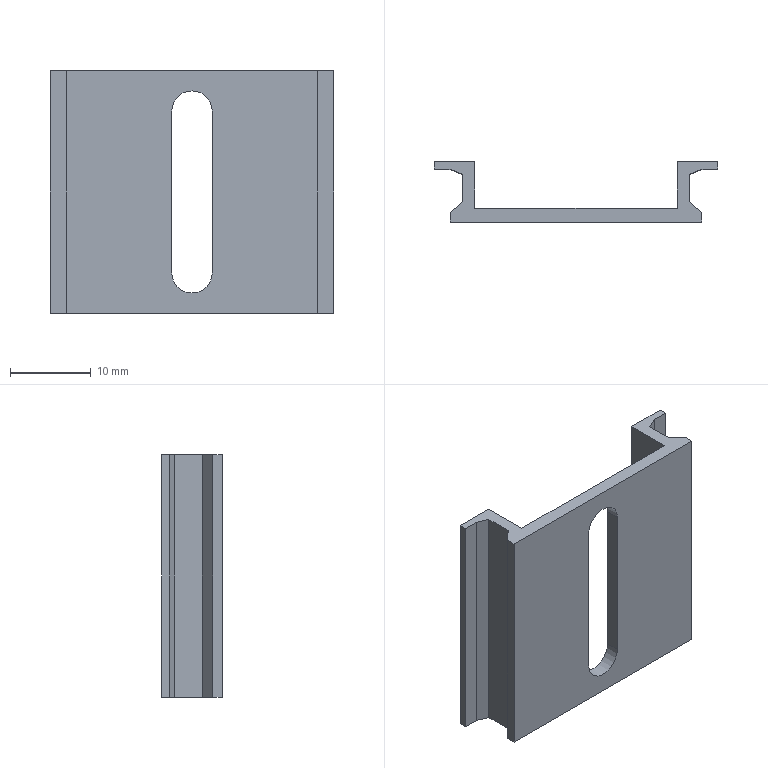Part | STEP file | Guide rail | 1 solid | 25 faces | box 35 x 7.5 x 30 mm | volume 2162 mm3 | plane 22 | cylinder 3 | commonest cylinder face diameters 5 x3
STEP:
#1=CARTESIAN_POINT('',(0.,0.,-87.5));
#2=VERTEX_POINT('',#1);
#3=CARTESIAN_POINT('',(2.5,0.,-90.));
#4=VERTEX_POINT('',#3);
#5=CARTESIAN_POINT('',(0.,0.,-90.));
#6=DIRECTION('',(0.,1.,0.));
#7=DIRECTION('',(0.,0.,1.));
#8=AXIS2_PLACEMENT_3D('',#5,#6,#7);
#9=CIRCLE('',#8,2.5);
#10=EDGE_CURVE('',#2,#4,#9,.T.);
#11=ORIENTED_EDGE('',*,*,#10,.F.);
#12=CARTESIAN_POINT('',(0.,1.7,-87.5));
#13=VERTEX_POINT('',#12);
#14=CARTESIAN_POINT('',(0.,-8.3,-87.5));
#15=DIRECTION('',(0.,1.,0.));
#16=VECTOR('',#15,1000.);
#17=LINE('',#14,#16);
#18=EDGE_CURVE('',#2,#13,#17,.T.);
#19=ORIENTED_EDGE('',*,*,#18,.T.);
#20=CARTESIAN_POINT('',(2.5,1.7,-90.));
#21=VERTEX_POINT('',#20);
#22=CARTESIAN_POINT('',(0.,1.7,-90.));
#23=DIRECTION('',(0.,1.,0.));
#24=DIRECTION('',(0.,0.,1.));
#25=AXIS2_PLACEMENT_3D('',#22,#23,#24);
#26=CIRCLE('',#25,2.5);
#27=EDGE_CURVE('',#13,#21,#26,.T.);
#28=ORIENTED_EDGE('',*,*,#27,.T.);
#29=CARTESIAN_POINT('',(2.5,-8.3,-90.));
#30=DIRECTION('',(0.,1.,0.));
#31=VECTOR('',#30,1000.);
#32=LINE('',#29,#31);
#33=EDGE_CURVE('',#4,#21,#32,.T.);
#34=ORIENTED_EDGE('',*,*,#33,.F.);
#35=EDGE_LOOP('',(#11,#19,#28,#34));
#36=FACE_OUTER_BOUND('',#35,.T.);
#37=CARTESIAN_POINT('',(0.,-8.3,-90.));
#38=DIRECTION('',(0.,1.,0.));
#39=DIRECTION('',(0.,0.,1.));
#40=AXIS2_PLACEMENT_3D('',#37,#38,#39);
#41=CYLINDRICAL_SURFACE('',#40,2.5);
#42=ADVANCED_FACE('',(#36),#41,.F.);
#43=CARTESIAN_POINT('',(14.05,5.9,-115.));
#44=VERTEX_POINT('',#43);
#45=CARTESIAN_POINT('',(14.05,5.9,-85.));
#46=VERTEX_POINT('',#45);
#47=CARTESIAN_POINT('',(14.05,5.9,58.));
#48=DIRECTION('',(0.,0.,1.));
#49=VECTOR('',#48,1000.);
#50=LINE('',#47,#49);
#51=EDGE_CURVE('',#44,#46,#50,.T.);
#52=ORIENTED_EDGE('',*,*,#51,.T.);
#53=CARTESIAN_POINT('',(14.05,2.5,-85.));
#54=VERTEX_POINT('',#53);
#55=CARTESIAN_POINT('',(14.05,0.,-85.));
#56=DIRECTION('',(0.,-1.,0.));
#57=VECTOR('',#56,1000.);
#58=LINE('',#55,#57);
#59=EDGE_CURVE('',#46,#54,#58,.T.);
#60=ORIENTED_EDGE('',*,*,#59,.T.);
#61=CARTESIAN_POINT('',(14.05,2.5,-115.));
#62=VERTEX_POINT('',#61);
#63=CARTESIAN_POINT('',(14.05,2.5,58.));
#64=DIRECTION('',(0.,0.,1.));
#65=VECTOR('',#64,1000.);
#66=LINE('',#63,#65);
#67=EDGE_CURVE('',#62,#54,#66,.T.);
#68=ORIENTED_EDGE('',*,*,#67,.F.);
#69=CARTESIAN_POINT('',(14.05,0.,-115.));
#70=DIRECTION('',(0.,1.,0.));
#71=VECTOR('',#70,1000.);
#72=LINE('',#69,#71);
#73=EDGE_CURVE('',#62,#44,#72,.T.);
#74=ORIENTED_EDGE('',*,*,#73,.T.);
#75=EDGE_LOOP('',(#52,#60,#68,#74));
#76=FACE_OUTER_BOUND('',#75,.T.);
#77=CARTESIAN_POINT('',(14.05,0.,58.));
#78=DIRECTION('',(-1.,0.,0.));
#79=DIRECTION('',(0.,0.,1.));
#80=AXIS2_PLACEMENT_3D('',#77,#78,#79);
#81=PLANE('',#80);
#82=ADVANCED_FACE('',(#76),#81,.F.);
#83=CARTESIAN_POINT('',(-14.05,2.5,-85.));
#84=VERTEX_POINT('',#83);
#85=CARTESIAN_POINT('',(-14.05,2.5,-115.));
#86=VERTEX_POINT('',#85);
#87=CARTESIAN_POINT('',(-14.05,2.5,58.));
#88=DIRECTION('',(0.,0.,-1.));
#89=VECTOR('',#88,1000.);
#90=LINE('',#87,#89);
#91=EDGE_CURVE('',#84,#86,#90,.T.);
#92=ORIENTED_EDGE('',*,*,#91,.F.);
#93=CARTESIAN_POINT('',(-14.05,5.9,-85.));
#94=VERTEX_POINT('',#93);
#95=CARTESIAN_POINT('',(-14.05,6.55,-85.));
#96=DIRECTION('',(0.,1.,0.));
#97=VECTOR('',#96,1000.);
#98=LINE('',#95,#97);
#99=EDGE_CURVE('',#84,#94,#98,.T.);
#100=ORIENTED_EDGE('',*,*,#99,.T.);
#101=CARTESIAN_POINT('',(-14.05,5.9,-115.));
#102=VERTEX_POINT('',#101);
#103=CARTESIAN_POINT('',(-14.05,5.9,-115.));
#104=DIRECTION('',(0.,0.,-1.));
#105=VECTOR('',#104,1000.);
#106=LINE('',#103,#105);
#107=EDGE_CURVE('',#94,#102,#106,.T.);
#108=ORIENTED_EDGE('',*,*,#107,.T.);
#109=CARTESIAN_POINT('',(-14.05,6.55,-115.));
#110=DIRECTION('',(0.,-1.,0.));
#111=VECTOR('',#110,1000.);
#112=LINE('',#109,#111);
#113=EDGE_CURVE('',#102,#86,#112,.T.);
#114=ORIENTED_EDGE('',*,*,#113,.T.);
#115=EDGE_LOOP('',(#92,#100,#108,#114));
#116=FACE_OUTER_BOUND('',#115,.T.);
#117=CARTESIAN_POINT('',(-14.05,6.55,58.));
#118=DIRECTION('',(1.,0.,0.));
#119=DIRECTION('',(0.,0.,-1.));
#120=AXIS2_PLACEMENT_3D('',#117,#118,#119);
#121=PLANE('',#120);
#122=ADVANCED_FACE('',(#116),#121,.F.);
#123=CARTESIAN_POINT('',(-2.5,1.7,-110.));
#124=VERTEX_POINT('',#123);
#125=CARTESIAN_POINT('',(-2.5,1.7,-90.));
#126=VERTEX_POINT('',#125);
#127=CARTESIAN_POINT('',(-2.5,1.7,-110.));
#128=DIRECTION('',(0.,0.,1.));
#129=VECTOR('',#128,1000.);
#130=LINE('',#127,#129);
#131=EDGE_CURVE('',#124,#126,#130,.T.);
#132=ORIENTED_EDGE('',*,*,#131,.F.);
#133=CARTESIAN_POINT('',(2.5,1.7,-110.));
#134=VERTEX_POINT('',#133);
#135=CARTESIAN_POINT('',(0.,1.7,-110.));
#136=DIRECTION('',(0.,1.,0.));
#137=DIRECTION('',(0.,0.,1.));
#138=AXIS2_PLACEMENT_3D('',#135,#136,#137);
#139=CIRCLE('',#138,2.5);
#140=EDGE_CURVE('',#134,#124,#139,.T.);
#141=ORIENTED_EDGE('',*,*,#140,.F.);
#142=CARTESIAN_POINT('',(2.5,1.7,-110.));
#143=DIRECTION('',(0.,0.,-1.));
#144=VECTOR('',#143,1000.);
#145=LINE('',#142,#144);
#146=EDGE_CURVE('',#21,#134,#145,.T.);
#147=ORIENTED_EDGE('',*,*,#146,.F.);
#148=ORIENTED_EDGE('',*,*,#27,.F.);
#149=CARTESIAN_POINT('',(0.,1.7,-90.));
#150=DIRECTION('',(0.,1.,0.));
#151=DIRECTION('',(0.,0.,1.));
#152=AXIS2_PLACEMENT_3D('',#149,#150,#151);
#153=CIRCLE('',#152,2.5);
#154=EDGE_CURVE('',#126,#13,#153,.T.);
#155=ORIENTED_EDGE('',*,*,#154,.F.);
#156=EDGE_LOOP('',(#132,#141,#147,#148,#155));
#157=FACE_BOUND('',#156,.T.);
#158=CARTESIAN_POINT('',(-12.5,1.7,-85.));
#159=VERTEX_POINT('',#158);
#160=CARTESIAN_POINT('',(-12.5,1.7,-115.));
#161=VERTEX_POINT('',#160);
#162=CARTESIAN_POINT('',(-12.5,1.7,-115.));
#163=DIRECTION('',(0.,0.,-1.));
#164=VECTOR('',#163,1000.);
#165=LINE('',#162,#164);
#166=EDGE_CURVE('',#159,#161,#165,.T.);
#167=ORIENTED_EDGE('',*,*,#166,.F.);
#168=CARTESIAN_POINT('',(12.5,1.7,-85.));
#169=VERTEX_POINT('',#168);
#170=CARTESIAN_POINT('',(12.5,1.7,-85.));
#171=DIRECTION('',(1.,0.,0.));
#172=VECTOR('',#171,1000.);
#173=LINE('',#170,#172);
#174=EDGE_CURVE('',#159,#169,#173,.T.);
#175=ORIENTED_EDGE('',*,*,#174,.T.);
#176=CARTESIAN_POINT('',(12.5,1.7,-115.));
#177=VERTEX_POINT('',#176);
#178=CARTESIAN_POINT('',(12.5,1.7,58.));
#179=DIRECTION('',(0.,0.,-1.));
#180=VECTOR('',#179,1000.);
#181=LINE('',#178,#180);
#182=EDGE_CURVE('',#169,#177,#181,.T.);
#183=ORIENTED_EDGE('',*,*,#182,.T.);
#184=CARTESIAN_POINT('',(12.5,1.7,-115.));
#185=DIRECTION('',(-1.,0.,0.));
#186=VECTOR('',#185,1000.);
#187=LINE('',#184,#186);
#188=EDGE_CURVE('',#177,#161,#187,.T.);
#189=ORIENTED_EDGE('',*,*,#188,.T.);
#190=EDGE_LOOP('',(#167,#175,#183,#189));
#191=FACE_OUTER_BOUND('',#190,.T.);
#192=CARTESIAN_POINT('',(12.5,1.7,58.));
#193=DIRECTION('',(0.,-1.,0.));
#194=DIRECTION('',(0.,0.,-1.));
#195=AXIS2_PLACEMENT_3D('',#192,#193,#194);
#196=PLANE('',#195);
#197=ADVANCED_FACE('',(#157,#191),#196,.F.);
#198=CARTESIAN_POINT('',(-17.5,7.5,-85.));
#199=VERTEX_POINT('',#198);
#200=CARTESIAN_POINT('',(-17.5,6.55,-85.));
#201=VERTEX_POINT('',#200);
#202=CARTESIAN_POINT('',(-17.5,0.,-85.));
#203=DIRECTION('',(0.,-1.,0.));
#204=VECTOR('',#203,1000.);
#205=LINE('',#202,#204);
#206=EDGE_CURVE('',#199,#201,#205,.T.);
#207=ORIENTED_EDGE('',*,*,#206,.F.);
#208=CARTESIAN_POINT('',(-17.5,7.5,-115.));
#209=VERTEX_POINT('',#208);
#210=CARTESIAN_POINT('',(-17.5,7.5,58.));
#211=DIRECTION('',(0.,0.,1.));
#212=VECTOR('',#211,1000.);
#213=LINE('',#210,#212);
#214=EDGE_CURVE('',#209,#199,#213,.T.);
#215=ORIENTED_EDGE('',*,*,#214,.F.);
#216=CARTESIAN_POINT('',(-17.5,6.55,-115.));
#217=VERTEX_POINT('',#216);
#218=CARTESIAN_POINT('',(-17.5,0.,-115.));
#219=DIRECTION('',(0.,1.,0.));
#220=VECTOR('',#219,1000.);
#221=LINE('',#218,#220);
#222=EDGE_CURVE('',#217,#209,#221,.T.);
#223=ORIENTED_EDGE('',*,*,#222,.F.);
#224=CARTESIAN_POINT('',(-17.5,6.55,58.));
#225=DIRECTION('',(0.,0.,-1.));
#226=VECTOR('',#225,1000.);
#227=LINE('',#224,#226);
#228=EDGE_CURVE('',#201,#217,#227,.T.);
#229=ORIENTED_EDGE('',*,*,#228,.F.);
#230=EDGE_LOOP('',(#207,#215,#223,#229));
#231=FACE_OUTER_BOUND('',#230,.T.);
#232=CARTESIAN_POINT('',(-17.5,0.,-115.));
#233=DIRECTION('',(-1.,0.,0.));
#234=DIRECTION('',(0.,0.,1.));
#235=AXIS2_PLACEMENT_3D('',#232,#233,#234);
#236=PLANE('',#235);
#237=ADVANCED_FACE('',(#231),#236,.T.);
#238=CARTESIAN_POINT('',(15.575,6.55,-115.));
#239=VERTEX_POINT('',#238);
#240=CARTESIAN_POINT('',(17.5,6.55,-115.));
#241=VERTEX_POINT('',#240);
#242=CARTESIAN_POINT('',(14.05,6.55,-115.));
#243=DIRECTION('',(1.,0.,0.));
#244=VECTOR('',#243,1000.);
#245=LINE('',#242,#244);
#246=EDGE_CURVE('',#239,#241,#245,.T.);
#247=ORIENTED_EDGE('',*,*,#246,.F.);
#248=CARTESIAN_POINT('',(15.575,6.55,-115.));
#249=DIRECTION('',(-0.9199,-0.3921,0.));
#250=VECTOR('',#249,1000.);
#251=LINE('',#248,#250);
#252=EDGE_CURVE('',#239,#44,#251,.T.);
#253=ORIENTED_EDGE('',*,*,#252,.T.);
#254=ORIENTED_EDGE('',*,*,#73,.F.);
#255=CARTESIAN_POINT('',(15.55,1.2,-115.));
#256=VERTEX_POINT('',#255);
#257=CARTESIAN_POINT('',(17.258,-0.2798,-115.));
#258=DIRECTION('',(-0.7557,0.6549,0.));
#259=VECTOR('',#258,1000.);
#260=LINE('',#257,#259);
#261=EDGE_CURVE('',#256,#62,#260,.T.);
#262=ORIENTED_EDGE('',*,*,#261,.F.);
#263=CARTESIAN_POINT('',(15.55,0.,-115.));
#264=VERTEX_POINT('',#263);
#265=CARTESIAN_POINT('',(15.55,1.2,-115.));
#266=DIRECTION('',(0.,1.,0.));
#267=VECTOR('',#266,1000.);
#268=LINE('',#265,#267);
#269=EDGE_CURVE('',#264,#256,#268,.T.);
#270=ORIENTED_EDGE('',*,*,#269,.F.);
#271=CARTESIAN_POINT('',(-15.55,0.,-115.));
#272=VERTEX_POINT('',#271);
#273=CARTESIAN_POINT('',(17.5,0.,-115.));
#274=DIRECTION('',(-1.,0.,0.));
#275=VECTOR('',#274,1000.);
#276=LINE('',#273,#275);
#277=EDGE_CURVE('',#264,#272,#276,.T.);
#278=ORIENTED_EDGE('',*,*,#277,.T.);
#279=CARTESIAN_POINT('',(-15.55,1.2,-115.));
#280=VERTEX_POINT('',#279);
#281=CARTESIAN_POINT('',(-15.55,0.,-115.));
#282=DIRECTION('',(0.,-1.,0.));
#283=VECTOR('',#282,1000.);
#284=LINE('',#281,#283);
#285=EDGE_CURVE('',#280,#272,#284,.T.);
#286=ORIENTED_EDGE('',*,*,#285,.F.);
#287=CARTESIAN_POINT('',(-15.55,1.2,-115.));
#288=DIRECTION('',(0.7557,0.6549,0.));
#289=VECTOR('',#288,1000.);
#290=LINE('',#287,#289);
#291=EDGE_CURVE('',#280,#86,#290,.T.);
#292=ORIENTED_EDGE('',*,*,#291,.T.);
#293=ORIENTED_EDGE('',*,*,#113,.F.);
#294=CARTESIAN_POINT('',(-15.574,6.55,-115.));
#295=VERTEX_POINT('',#294);
#296=CARTESIAN_POINT('',(-14.05,5.9,-115.));
#297=DIRECTION('',(-0.9199,0.3921,0.));
#298=VECTOR('',#297,1000.);
#299=LINE('',#296,#298);
#300=EDGE_CURVE('',#102,#295,#299,.T.);
#301=ORIENTED_EDGE('',*,*,#300,.T.);
#302=CARTESIAN_POINT('',(-17.5,6.55,-115.));
#303=DIRECTION('',(1.,0.,0.));
#304=VECTOR('',#303,1000.);
#305=LINE('',#302,#304);
#306=EDGE_CURVE('',#217,#295,#305,.T.);
#307=ORIENTED_EDGE('',*,*,#306,.F.);
#308=ORIENTED_EDGE('',*,*,#222,.T.);
#309=CARTESIAN_POINT('',(-12.5,7.5,-115.));
#310=VERTEX_POINT('',#309);
#311=CARTESIAN_POINT('',(-17.5,7.5,-115.));
#312=DIRECTION('',(-1.,0.,0.));
#313=VECTOR('',#312,1000.);
#314=LINE('',#311,#313);
#315=EDGE_CURVE('',#310,#209,#314,.T.);
#316=ORIENTED_EDGE('',*,*,#315,.F.);
#317=CARTESIAN_POINT('',(-12.5,7.5,-115.));
#318=DIRECTION('',(0.,-1.,0.));
#319=VECTOR('',#318,1000.);
#320=LINE('',#317,#319);
#321=EDGE_CURVE('',#310,#161,#320,.T.);
#322=ORIENTED_EDGE('',*,*,#321,.T.);
#323=ORIENTED_EDGE('',*,*,#188,.F.);
#324=CARTESIAN_POINT('',(12.5,7.5,-115.));
#325=VERTEX_POINT('',#324);
#326=CARTESIAN_POINT('',(12.5,7.5,-115.));
#327=DIRECTION('',(0.,-1.,0.));
#328=VECTOR('',#327,1000.);
#329=LINE('',#326,#328);
#330=EDGE_CURVE('',#325,#177,#329,.T.);
#331=ORIENTED_EDGE('',*,*,#330,.F.);
#332=CARTESIAN_POINT('',(17.5,7.5,-115.));
#333=VERTEX_POINT('',#332);
#334=CARTESIAN_POINT('',(17.5,7.5,-115.));
#335=DIRECTION('',(-1.,0.,0.));
#336=VECTOR('',#335,1000.);
#337=LINE('',#334,#336);
#338=EDGE_CURVE('',#333,#325,#337,.T.);
#339=ORIENTED_EDGE('',*,*,#338,.F.);
#340=CARTESIAN_POINT('',(17.5,0.,-115.));
#341=DIRECTION('',(0.,1.,0.));
#342=VECTOR('',#341,1000.);
#343=LINE('',#340,#342);
#344=EDGE_CURVE('',#241,#333,#343,.T.);
#345=ORIENTED_EDGE('',*,*,#344,.F.);
#346=EDGE_LOOP('',(#247,#253,#254,#262,#270,#278,#286,#292,#293,#301,#307,#308,#316,#322,#323,#331,#339,#345));
#347=FACE_OUTER_BOUND('',#346,.T.);
#348=CARTESIAN_POINT('',(17.5,0.,-115.));
#349=DIRECTION('',(0.,0.,-1.));
#350=DIRECTION('',(-1.,0.,0.));
#351=AXIS2_PLACEMENT_3D('',#348,#349,#350);
#352=PLANE('',#351);
#353=ADVANCED_FACE('',(#347),#352,.T.);
#354=CARTESIAN_POINT('',(17.5,6.55,-85.));
#355=VERTEX_POINT('',#354);
#356=CARTESIAN_POINT('',(17.5,7.5,-85.));
#357=VERTEX_POINT('',#356);
#358=CARTESIAN_POINT('',(17.5,0.,-85.));
#359=DIRECTION('',(0.,1.,0.));
#360=VECTOR('',#359,1000.);
#361=LINE('',#358,#360);
#362=EDGE_CURVE('',#355,#357,#361,.T.);
#363=ORIENTED_EDGE('',*,*,#362,.F.);
#364=CARTESIAN_POINT('',(17.5,6.55,58.));
#365=DIRECTION('',(0.,0.,-1.));
#366=VECTOR('',#365,1000.);
#367=LINE('',#364,#366);
#368=EDGE_CURVE('',#355,#241,#367,.T.);
#369=ORIENTED_EDGE('',*,*,#368,.T.);
#370=ORIENTED_EDGE('',*,*,#344,.T.);
#371=CARTESIAN_POINT('',(17.5,7.5,58.));
#372=DIRECTION('',(0.,0.,-1.));
#373=VECTOR('',#372,1000.);
#374=LINE('',#371,#373);
#375=EDGE_CURVE('',#357,#333,#374,.T.);
#376=ORIENTED_EDGE('',*,*,#375,.F.);
#377=EDGE_LOOP('',(#363,#369,#370,#376));
#378=FACE_OUTER_BOUND('',#377,.T.);
#379=CARTESIAN_POINT('',(17.5,0.,58.));
#380=DIRECTION('',(1.,0.,0.));
#381=DIRECTION('',(0.,0.,-1.));
#382=AXIS2_PLACEMENT_3D('',#379,#380,#381);
#383=PLANE('',#382);
#384=ADVANCED_FACE('',(#378),#383,.T.);
#385=CARTESIAN_POINT('',(2.5,0.,-110.));
#386=VERTEX_POINT('',#385);
#387=CARTESIAN_POINT('',(2.5,0.,58.));
#388=DIRECTION('',(0.,0.,-1.));
#389=VECTOR('',#388,1000.);
#390=LINE('',#387,#389);
#391=EDGE_CURVE('',#4,#386,#390,.T.);
#392=ORIENTED_EDGE('',*,*,#391,.T.);
#393=CARTESIAN_POINT('',(-2.5,0.,-110.));
#394=VERTEX_POINT('',#393);
#395=CARTESIAN_POINT('',(0.,0.,-110.));
#396=DIRECTION('',(0.,1.,0.));
#397=DIRECTION('',(0.,0.,1.));
#398=AXIS2_PLACEMENT_3D('',#395,#396,#397);
#399=CIRCLE('',#398,2.5);
#400=EDGE_CURVE('',#386,#394,#399,.T.);
#401=ORIENTED_EDGE('',*,*,#400,.T.);
#402=CARTESIAN_POINT('',(-2.5,0.,-90.));
#403=VERTEX_POINT('',#402);
#404=CARTESIAN_POINT('',(-2.5,0.,58.));
#405=DIRECTION('',(0.,0.,1.));
#406=VECTOR('',#405,1000.);
#407=LINE('',#404,#406);
#408=EDGE_CURVE('',#394,#403,#407,.T.);
#409=ORIENTED_EDGE('',*,*,#408,.T.);
#410=CARTESIAN_POINT('',(0.,0.,-90.));
#411=DIRECTION('',(0.,1.,0.));
#412=DIRECTION('',(0.,0.,1.));
#413=AXIS2_PLACEMENT_3D('',#410,#411,#412);
#414=CIRCLE('',#413,2.5);
#415=EDGE_CURVE('',#403,#2,#414,.T.);
#416=ORIENTED_EDGE('',*,*,#415,.T.);
#417=ORIENTED_EDGE('',*,*,#10,.T.);
#418=EDGE_LOOP('',(#392,#401,#409,#416,#417));
#419=FACE_BOUND('',#418,.T.);
#420=CARTESIAN_POINT('',(15.55,0.,-85.));
#421=VERTEX_POINT('',#420);
#422=CARTESIAN_POINT('',(15.55,0.,-115.));
#423=DIRECTION('',(0.,0.,-1.));
#424=VECTOR('',#423,1000.);
#425=LINE('',#422,#424);
#426=EDGE_CURVE('',#421,#264,#425,.T.);
#427=ORIENTED_EDGE('',*,*,#426,.F.);
#428=CARTESIAN_POINT('',(-15.55,0.,-85.));
#429=VERTEX_POINT('',#428);
#430=CARTESIAN_POINT('',(-17.5,0.,-85.));
#431=DIRECTION('',(-1.,0.,0.));
#432=VECTOR('',#431,1000.);
#433=LINE('',#430,#432);
#434=EDGE_CURVE('',#421,#429,#433,.T.);
#435=ORIENTED_EDGE('',*,*,#434,.T.);
#436=CARTESIAN_POINT('',(-15.55,0.,58.));
#437=DIRECTION('',(0.,0.,1.));
#438=VECTOR('',#437,1000.);
#439=LINE('',#436,#438);
#440=EDGE_CURVE('',#272,#429,#439,.T.);
#441=ORIENTED_EDGE('',*,*,#440,.F.);
#442=ORIENTED_EDGE('',*,*,#277,.F.);
#443=EDGE_LOOP('',(#427,#435,#441,#442));
#444=FACE_OUTER_BOUND('',#443,.T.);
#445=CARTESIAN_POINT('',(-17.5,0.,58.));
#446=DIRECTION('',(0.,1.,0.));
#447=DIRECTION('',(0.,0.,1.));
#448=AXIS2_PLACEMENT_3D('',#445,#446,#447);
#449=PLANE('',#448);
#450=ADVANCED_FACE('',(#419,#444),#449,.F.);
#451=CARTESIAN_POINT('',(12.5,7.5,-85.));
#452=VERTEX_POINT('',#451);
#453=CARTESIAN_POINT('',(-17.5,7.5,-85.));
#454=DIRECTION('',(-1.,0.,0.));
#455=VECTOR('',#454,1000.);
#456=LINE('',#453,#455);
#457=EDGE_CURVE('',#357,#452,#456,.T.);
#458=ORIENTED_EDGE('',*,*,#457,.F.);
#459=ORIENTED_EDGE('',*,*,#375,.T.);
#460=ORIENTED_EDGE('',*,*,#338,.T.);
#461=CARTESIAN_POINT('',(12.5,7.5,58.));
#462=DIRECTION('',(0.,0.,-1.));
#463=VECTOR('',#462,1000.);
#464=LINE('',#461,#463);
#465=EDGE_CURVE('',#452,#325,#464,.T.);
#466=ORIENTED_EDGE('',*,*,#465,.F.);
#467=EDGE_LOOP('',(#458,#459,#460,#466));
#468=FACE_OUTER_BOUND('',#467,.T.);
#469=CARTESIAN_POINT('',(-17.5,7.5,58.));
#470=DIRECTION('',(0.,1.,0.));
#471=DIRECTION('',(0.,0.,1.));
#472=AXIS2_PLACEMENT_3D('',#469,#470,#471);
#473=PLANE('',#472);
#474=ADVANCED_FACE('',(#468),#473,.T.);
#475=ORIENTED_EDGE('',*,*,#182,.F.);
#476=CARTESIAN_POINT('',(12.5,7.5,-85.));
#477=DIRECTION('',(0.,1.,0.));
#478=VECTOR('',#477,1000.);
#479=LINE('',#476,#478);
#480=EDGE_CURVE('',#169,#452,#479,.T.);
#481=ORIENTED_EDGE('',*,*,#480,.T.);
#482=ORIENTED_EDGE('',*,*,#465,.T.);
#483=ORIENTED_EDGE('',*,*,#330,.T.);
#484=EDGE_LOOP('',(#475,#481,#482,#483));
#485=FACE_OUTER_BOUND('',#484,.T.);
#486=CARTESIAN_POINT('',(12.5,7.5,58.));
#487=DIRECTION('',(1.,0.,0.));
#488=DIRECTION('',(0.,1.,0.));
#489=AXIS2_PLACEMENT_3D('',#486,#487,#488);
#490=PLANE('',#489);
#491=ADVANCED_FACE('',(#485),#490,.F.);
#492=CARTESIAN_POINT('',(-12.5,7.5,-85.));
#493=VERTEX_POINT('',#492);
#494=CARTESIAN_POINT('',(-12.5,7.5,-115.));
#495=DIRECTION('',(0.,0.,-1.));
#496=VECTOR('',#495,1000.);
#497=LINE('',#494,#496);
#498=EDGE_CURVE('',#493,#310,#497,.T.);
#499=ORIENTED_EDGE('',*,*,#498,.F.);
#500=CARTESIAN_POINT('',(-12.5,7.5,-85.));
#501=DIRECTION('',(0.,-1.,0.));
#502=VECTOR('',#501,1000.);
#503=LINE('',#500,#502);
#504=EDGE_CURVE('',#493,#159,#503,.T.);
#505=ORIENTED_EDGE('',*,*,#504,.T.);
#506=ORIENTED_EDGE('',*,*,#166,.T.);
#507=ORIENTED_EDGE('',*,*,#321,.F.);
#508=EDGE_LOOP('',(#499,#505,#506,#507));
#509=FACE_OUTER_BOUND('',#508,.T.);
#510=CARTESIAN_POINT('',(-12.5,7.5,-115.));
#511=DIRECTION('',(-1.,0.,0.));
#512=DIRECTION('',(0.,0.,1.));
#513=AXIS2_PLACEMENT_3D('',#510,#511,#512);
#514=PLANE('',#513);
#515=ADVANCED_FACE('',(#509),#514,.F.);
#516=ORIENTED_EDGE('',*,*,#214,.T.);
#517=CARTESIAN_POINT('',(-17.5,7.5,-85.));
#518=DIRECTION('',(1.,0.,0.));
#519=VECTOR('',#518,1000.);
#520=LINE('',#517,#519);
#521=EDGE_CURVE('',#199,#493,#520,.T.);
#522=ORIENTED_EDGE('',*,*,#521,.T.);
#523=ORIENTED_EDGE('',*,*,#498,.T.);
#524=ORIENTED_EDGE('',*,*,#315,.T.);
#525=EDGE_LOOP('',(#516,#522,#523,#524));
#526=FACE_OUTER_BOUND('',#525,.T.);
#527=CARTESIAN_POINT('',(-17.5,7.5,58.));
#528=DIRECTION('',(0.,-1.,0.));
#529=DIRECTION('',(0.,0.,-1.));
#530=AXIS2_PLACEMENT_3D('',#527,#528,#529);
#531=PLANE('',#530);
#532=ADVANCED_FACE('',(#526),#531,.F.);
#533=CARTESIAN_POINT('',(-15.574,6.55,-85.));
#534=VERTEX_POINT('',#533);
#535=CARTESIAN_POINT('',(-15.574,6.55,58.));
#536=DIRECTION('',(0.,0.,1.));
#537=VECTOR('',#536,1000.);
#538=LINE('',#535,#537);
#539=EDGE_CURVE('',#295,#534,#538,.T.);
#540=ORIENTED_EDGE('',*,*,#539,.T.);
#541=CARTESIAN_POINT('',(-17.5,6.55,-85.));
#542=DIRECTION('',(-1.,0.,0.));
#543=VECTOR('',#542,1000.);
#544=LINE('',#541,#543);
#545=EDGE_CURVE('',#534,#201,#544,.T.);
#546=ORIENTED_EDGE('',*,*,#545,.T.);
#547=ORIENTED_EDGE('',*,*,#228,.T.);
#548=ORIENTED_EDGE('',*,*,#306,.T.);
#549=EDGE_LOOP('',(#540,#546,#547,#548));
#550=FACE_OUTER_BOUND('',#549,.T.);
#551=CARTESIAN_POINT('',(-17.5,6.55,58.));
#552=DIRECTION('',(0.,1.,0.));
#553=DIRECTION('',(-1.,0.,0.));
#554=AXIS2_PLACEMENT_3D('',#551,#552,#553);
#555=PLANE('',#554);
#556=ADVANCED_FACE('',(#550),#555,.F.);
#557=CARTESIAN_POINT('',(-15.55,1.2,-85.));
#558=VERTEX_POINT('',#557);
#559=CARTESIAN_POINT('',(-15.55,1.2,-115.));
#560=DIRECTION('',(0.,0.,-1.));
#561=VECTOR('',#560,1000.);
#562=LINE('',#559,#561);
#563=EDGE_CURVE('',#558,#280,#562,.T.);
#564=ORIENTED_EDGE('',*,*,#563,.F.);
#565=CARTESIAN_POINT('',(-15.55,1.2,-85.));
#566=DIRECTION('',(0.7557,0.6549,0.));
#567=VECTOR('',#566,1000.);
#568=LINE('',#565,#567);
#569=EDGE_CURVE('',#558,#84,#568,.T.);
#570=ORIENTED_EDGE('',*,*,#569,.T.);
#571=ORIENTED_EDGE('',*,*,#91,.T.);
#572=ORIENTED_EDGE('',*,*,#291,.F.);
#573=EDGE_LOOP('',(#564,#570,#571,#572));
#574=FACE_OUTER_BOUND('',#573,.T.);
#575=CARTESIAN_POINT('',(-15.55,1.2,-115.));
#576=DIRECTION('',(-0.6549,0.7557,0.));
#577=DIRECTION('',(-0.7557,-0.6549,0.));
#578=AXIS2_PLACEMENT_3D('',#575,#576,#577);
#579=PLANE('',#578);
#580=ADVANCED_FACE('',(#574),#579,.T.);
#581=ORIENTED_EDGE('',*,*,#440,.T.);
#582=CARTESIAN_POINT('',(-15.55,0.,-85.));
#583=DIRECTION('',(0.,1.,0.));
#584=VECTOR('',#583,1000.);
#585=LINE('',#582,#584);
#586=EDGE_CURVE('',#429,#558,#585,.T.);
#587=ORIENTED_EDGE('',*,*,#586,.T.);
#588=ORIENTED_EDGE('',*,*,#563,.T.);
#589=ORIENTED_EDGE('',*,*,#285,.T.);
#590=EDGE_LOOP('',(#581,#587,#588,#589));
#591=FACE_OUTER_BOUND('',#590,.T.);
#592=CARTESIAN_POINT('',(-15.55,0.,58.));
#593=DIRECTION('',(1.,0.,0.));
#594=DIRECTION('',(0.,0.,-1.));
#595=AXIS2_PLACEMENT_3D('',#592,#593,#594);
#596=PLANE('',#595);
#597=ADVANCED_FACE('',(#591),#596,.F.);
#598=ORIENTED_EDGE('',*,*,#368,.F.);
#599=CARTESIAN_POINT('',(15.575,6.55,-85.));
#600=VERTEX_POINT('',#599);
#601=CARTESIAN_POINT('',(14.05,6.55,-85.));
#602=DIRECTION('',(-1.,0.,0.));
#603=VECTOR('',#602,1000.);
#604=LINE('',#601,#603);
#605=EDGE_CURVE('',#355,#600,#604,.T.);
#606=ORIENTED_EDGE('',*,*,#605,.T.);
#607=CARTESIAN_POINT('',(15.575,6.55,-115.));
#608=DIRECTION('',(0.,0.,-1.));
#609=VECTOR('',#608,1000.);
#610=LINE('',#607,#609);
#611=EDGE_CURVE('',#600,#239,#610,.T.);
#612=ORIENTED_EDGE('',*,*,#611,.T.);
#613=ORIENTED_EDGE('',*,*,#246,.T.);
#614=EDGE_LOOP('',(#598,#606,#612,#613));
#615=FACE_OUTER_BOUND('',#614,.T.);
#616=CARTESIAN_POINT('',(14.05,6.55,58.));
#617=DIRECTION('',(0.,1.,0.));
#618=DIRECTION('',(-1.,0.,0.));
#619=AXIS2_PLACEMENT_3D('',#616,#617,#618);
#620=PLANE('',#619);
#621=ADVANCED_FACE('',(#615),#620,.F.);
#622=ORIENTED_EDGE('',*,*,#67,.T.);
#623=CARTESIAN_POINT('',(15.55,1.2,-85.));
#624=VERTEX_POINT('',#623);
#625=CARTESIAN_POINT('',(15.55,1.2,-85.));
#626=DIRECTION('',(0.7557,-0.6549,0.));
#627=VECTOR('',#626,1000.);
#628=LINE('',#625,#627);
#629=EDGE_CURVE('',#54,#624,#628,.T.);
#630=ORIENTED_EDGE('',*,*,#629,.T.);
#631=CARTESIAN_POINT('',(15.55,1.2,58.));
#632=DIRECTION('',(0.,0.,1.));
#633=VECTOR('',#632,1000.);
#634=LINE('',#631,#633);
#635=EDGE_CURVE('',#256,#624,#634,.T.);
#636=ORIENTED_EDGE('',*,*,#635,.F.);
#637=ORIENTED_EDGE('',*,*,#261,.T.);
#638=EDGE_LOOP('',(#622,#630,#636,#637));
#639=FACE_OUTER_BOUND('',#638,.T.);
#640=CARTESIAN_POINT('',(15.55,1.2,58.));
#641=DIRECTION('',(0.6549,0.7557,0.));
#642=DIRECTION('',(-0.7557,0.6549,0.));
#643=AXIS2_PLACEMENT_3D('',#640,#641,#642);
#644=PLANE('',#643);
#645=ADVANCED_FACE('',(#639),#644,.T.);
#646=ORIENTED_EDGE('',*,*,#635,.T.);
#647=CARTESIAN_POINT('',(15.55,1.2,-85.));
#648=DIRECTION('',(0.,-1.,0.));
#649=VECTOR('',#648,1000.);
#650=LINE('',#647,#649);
#651=EDGE_CURVE('',#624,#421,#650,.T.);
#652=ORIENTED_EDGE('',*,*,#651,.T.);
#653=ORIENTED_EDGE('',*,*,#426,.T.);
#654=ORIENTED_EDGE('',*,*,#269,.T.);
#655=EDGE_LOOP('',(#646,#652,#653,#654));
#656=FACE_OUTER_BOUND('',#655,.T.);
#657=CARTESIAN_POINT('',(15.55,1.2,58.));
#658=DIRECTION('',(-1.,0.,0.));
#659=DIRECTION('',(0.,0.,1.));
#660=AXIS2_PLACEMENT_3D('',#657,#658,#659);
#661=PLANE('',#660);
#662=ADVANCED_FACE('',(#656),#661,.F.);
#663=ORIENTED_EDGE('',*,*,#107,.F.);
#664=CARTESIAN_POINT('',(-14.05,5.9,-85.));
#665=DIRECTION('',(-0.9199,0.3921,0.));
#666=VECTOR('',#665,1000.);
#667=LINE('',#664,#666);
#668=EDGE_CURVE('',#94,#534,#667,.T.);
#669=ORIENTED_EDGE('',*,*,#668,.T.);
#670=ORIENTED_EDGE('',*,*,#539,.F.);
#671=ORIENTED_EDGE('',*,*,#300,.F.);
#672=EDGE_LOOP('',(#663,#669,#670,#671));
#673=FACE_OUTER_BOUND('',#672,.T.);
#674=CARTESIAN_POINT('',(-14.05,5.9,58.));
#675=DIRECTION('',(-0.3921,-0.9199,0.));
#676=DIRECTION('',(0.9199,-0.3921,0.));
#677=AXIS2_PLACEMENT_3D('',#674,#675,#676);
#678=PLANE('',#677);
#679=ADVANCED_FACE('',(#673),#678,.T.);
#680=ORIENTED_EDGE('',*,*,#611,.F.);
#681=CARTESIAN_POINT('',(15.575,6.55,-85.));
#682=DIRECTION('',(-0.9199,-0.3921,0.));
#683=VECTOR('',#682,1000.);
#684=LINE('',#681,#683);
#685=EDGE_CURVE('',#600,#46,#684,.T.);
#686=ORIENTED_EDGE('',*,*,#685,.T.);
#687=ORIENTED_EDGE('',*,*,#51,.F.);
#688=ORIENTED_EDGE('',*,*,#252,.F.);
#689=EDGE_LOOP('',(#680,#686,#687,#688));
#690=FACE_OUTER_BOUND('',#689,.T.);
#691=CARTESIAN_POINT('',(15.575,6.55,58.));
#692=DIRECTION('',(0.3921,-0.9199,0.));
#693=DIRECTION('',(0.9199,0.3921,0.));
#694=AXIS2_PLACEMENT_3D('',#691,#692,#693);
#695=PLANE('',#694);
#696=ADVANCED_FACE('',(#690),#695,.T.);
#697=ORIENTED_EDGE('',*,*,#206,.T.);
#698=ORIENTED_EDGE('',*,*,#545,.F.);
#699=ORIENTED_EDGE('',*,*,#668,.F.);
#700=ORIENTED_EDGE('',*,*,#99,.F.);
#701=ORIENTED_EDGE('',*,*,#569,.F.);
#702=ORIENTED_EDGE('',*,*,#586,.F.);
#703=ORIENTED_EDGE('',*,*,#434,.F.);
#704=ORIENTED_EDGE('',*,*,#651,.F.);
#705=ORIENTED_EDGE('',*,*,#629,.F.);
#706=ORIENTED_EDGE('',*,*,#59,.F.);
#707=ORIENTED_EDGE('',*,*,#685,.F.);
#708=ORIENTED_EDGE('',*,*,#605,.F.);
#709=ORIENTED_EDGE('',*,*,#362,.T.);
#710=ORIENTED_EDGE('',*,*,#457,.T.);
#711=ORIENTED_EDGE('',*,*,#480,.F.);
#712=ORIENTED_EDGE('',*,*,#174,.F.);
#713=ORIENTED_EDGE('',*,*,#504,.F.);
#714=ORIENTED_EDGE('',*,*,#521,.F.);
#715=EDGE_LOOP('',(#697,#698,#699,#700,#701,#702,#703,#704,#705,#706,#707,#708,#709,#710,#711,#712,#713,#714));
#716=FACE_OUTER_BOUND('',#715,.T.);
#717=CARTESIAN_POINT('',(-26.173,-10.5,-85.));
#718=DIRECTION('',(0.,0.,-1.));
#719=DIRECTION('',(-1.,0.,0.));
#720=AXIS2_PLACEMENT_3D('',#717,#718,#719);
#721=PLANE('',#720);
#722=ADVANCED_FACE('',(#716),#721,.F.);
#723=CARTESIAN_POINT('',(2.5,-8.3,-110.));
#724=DIRECTION('',(0.,1.,0.));
#725=VECTOR('',#724,1000.);
#726=LINE('',#723,#725);
#727=EDGE_CURVE('',#386,#134,#726,.T.);
#728=ORIENTED_EDGE('',*,*,#727,.T.);
#729=ORIENTED_EDGE('',*,*,#140,.T.);
#730=CARTESIAN_POINT('',(-2.5,-8.3,-110.));
#731=DIRECTION('',(0.,1.,0.));
#732=VECTOR('',#731,1000.);
#733=LINE('',#730,#732);
#734=EDGE_CURVE('',#394,#124,#733,.T.);
#735=ORIENTED_EDGE('',*,*,#734,.F.);
#736=ORIENTED_EDGE('',*,*,#400,.F.);
#737=EDGE_LOOP('',(#728,#729,#735,#736));
#738=FACE_OUTER_BOUND('',#737,.T.);
#739=CARTESIAN_POINT('',(0.,-8.3,-110.));
#740=DIRECTION('',(0.,1.,0.));
#741=DIRECTION('',(0.,0.,1.));
#742=AXIS2_PLACEMENT_3D('',#739,#740,#741);
#743=CYLINDRICAL_SURFACE('',#742,2.5);
#744=ADVANCED_FACE('',(#738),#743,.F.);
#745=ORIENTED_EDGE('',*,*,#33,.T.);
#746=ORIENTED_EDGE('',*,*,#146,.T.);
#747=ORIENTED_EDGE('',*,*,#727,.F.);
#748=ORIENTED_EDGE('',*,*,#391,.F.);
#749=EDGE_LOOP('',(#745,#746,#747,#748));
#750=FACE_OUTER_BOUND('',#749,.T.);
#751=CARTESIAN_POINT('',(2.5,-8.3,-110.));
#752=DIRECTION('',(1.,0.,0.));
#753=DIRECTION('',(0.,0.,-1.));
#754=AXIS2_PLACEMENT_3D('',#751,#752,#753);
#755=PLANE('',#754);
#756=ADVANCED_FACE('',(#750),#755,.F.);
#757=ORIENTED_EDGE('',*,*,#18,.F.);
#758=ORIENTED_EDGE('',*,*,#415,.F.);
#759=CARTESIAN_POINT('',(-2.5,-8.3,-90.));
#760=DIRECTION('',(0.,1.,0.));
#761=VECTOR('',#760,1000.);
#762=LINE('',#759,#761);
#763=EDGE_CURVE('',#403,#126,#762,.T.);
#764=ORIENTED_EDGE('',*,*,#763,.T.);
#765=ORIENTED_EDGE('',*,*,#154,.T.);
#766=EDGE_LOOP('',(#757,#758,#764,#765));
#767=FACE_OUTER_BOUND('',#766,.T.);
#768=CARTESIAN_POINT('',(0.,-8.3,-90.));
#769=DIRECTION('',(0.,1.,0.));
#770=DIRECTION('',(0.,0.,1.));
#771=AXIS2_PLACEMENT_3D('',#768,#769,#770);
#772=CYLINDRICAL_SURFACE('',#771,2.5);
#773=ADVANCED_FACE('',(#767),#772,.F.);
#774=ORIENTED_EDGE('',*,*,#734,.T.);
#775=ORIENTED_EDGE('',*,*,#131,.T.);
#776=ORIENTED_EDGE('',*,*,#763,.F.);
#777=ORIENTED_EDGE('',*,*,#408,.F.);
#778=EDGE_LOOP('',(#774,#775,#776,#777));
#779=FACE_OUTER_BOUND('',#778,.T.);
#780=CARTESIAN_POINT('',(-2.5,-8.3,-110.));
#781=DIRECTION('',(-1.,0.,0.));
#782=DIRECTION('',(0.,0.,1.));
#783=AXIS2_PLACEMENT_3D('',#780,#781,#782);
#784=PLANE('',#783);
#785=ADVANCED_FACE('',(#779),#784,.F.);
#786=CLOSED_SHELL('',(#42,#82,#122,#197,#237,#353,#384,#450,#474,#491,#515,#532,#556,#580,#597,#621,#645,#662,#679,#696,#722,#744,#756,#773,#785));
#787=MANIFOLD_SOLID_BREP('',#786);
#788=CARTESIAN_POINT('',(0.,0.,0.));
#789=DIRECTION('',(0.,0.,1.));
#790=DIRECTION('',(1.,0.,0.));
#791=AXIS2_PLACEMENT_3D('',#788,#789,#790);
#792=(LENGTH_UNIT()NAMED_UNIT(*)SI_UNIT(.MILLI.,.METRE.));
#793=UNCERTAINTY_MEASURE_WITH_UNIT(LENGTH_MEASURE(0.00001),#792,'','');
#794=(NAMED_UNIT(*)PLANE_ANGLE_UNIT()SI_UNIT($,.RADIAN.));
#795=(NAMED_UNIT(*)SI_UNIT($,.STERADIAN.)SOLID_ANGLE_UNIT());
#796=(GEOMETRIC_REPRESENTATION_CONTEXT(3)GLOBAL_UNCERTAINTY_ASSIGNED_CONTEXT((#793))GLOBAL_UNIT_ASSIGNED_CONTEXT((#792,#794,#795))REPRESENTATION_CONTEXT('',''));
#797=ADVANCED_BREP_SHAPE_REPRESENTATION('',(#787,#791),#796);